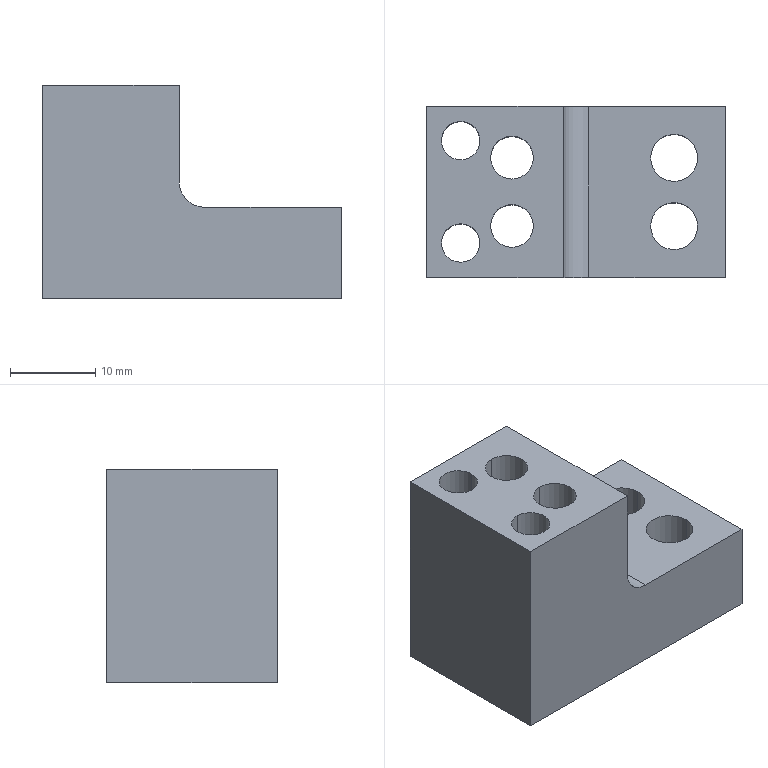Part | NX | 1 solid | 21 faces | box 35 x 20 x 25 mm | volume 9819 mm3 | cylinder 13 | plane 8 | commonest cylinder face diameters 4.5 x4 5 x4 5.5 x4 6 x1
STEP:
#1=CARTESIAN_POINT('',(0.,-20.,0.));
#2=VERTEX_POINT('',#1);
#3=CARTESIAN_POINT('',(0.,0.,0.));
#4=VERTEX_POINT('',#3);
#5=CARTESIAN_POINT('',(0.,0.,0.));
#6=DIRECTION('',(0.,1.,0.));
#7=VECTOR('',#6,1000.);
#8=LINE('',#5,#7);
#9=EDGE_CURVE('',#2,#4,#8,.T.);
#10=ORIENTED_EDGE('',*,*,#9,.T.);
#11=CARTESIAN_POINT('',(35.,0.,0.));
#12=VERTEX_POINT('',#11);
#13=CARTESIAN_POINT('',(0.,0.,0.));
#14=DIRECTION('',(1.,0.,0.));
#15=VECTOR('',#14,1000.);
#16=LINE('',#13,#15);
#17=EDGE_CURVE('',#4,#12,#16,.T.);
#18=ORIENTED_EDGE('',*,*,#17,.T.);
#19=CARTESIAN_POINT('',(35.,-20.,0.));
#20=VERTEX_POINT('',#19);
#21=CARTESIAN_POINT('',(35.,0.,0.));
#22=DIRECTION('',(0.,-1.,0.));
#23=VECTOR('',#22,1000.);
#24=LINE('',#21,#23);
#25=EDGE_CURVE('',#12,#20,#24,.T.);
#26=ORIENTED_EDGE('',*,*,#25,.T.);
#27=CARTESIAN_POINT('',(0.,-20.,0.));
#28=DIRECTION('',(-1.,0.,0.));
#29=VECTOR('',#28,1000.);
#30=LINE('',#27,#29);
#31=EDGE_CURVE('',#20,#2,#30,.T.);
#32=ORIENTED_EDGE('',*,*,#31,.T.);
#33=EDGE_LOOP('',(#10,#18,#26,#32));
#34=FACE_BOUND('',#33,.T.);
#35=CARTESIAN_POINT('',(6.25,-4.,0.));
#36=VERTEX_POINT('',#35);
#37=CARTESIAN_POINT('',(1.75,-4.,0.));
#38=VERTEX_POINT('',#37);
#39=CARTESIAN_POINT('',(4.,-4.,0.));
#40=DIRECTION('',(0.,0.,1.));
#41=DIRECTION('',(1.,0.,0.));
#42=AXIS2_PLACEMENT_3D('',#39,#40,#41);
#43=CIRCLE('',#42,2.25);
#44=EDGE_CURVE('',#36,#38,#43,.T.);
#45=ORIENTED_EDGE('',*,*,#44,.T.);
#46=CARTESIAN_POINT('',(4.,-4.,0.));
#47=DIRECTION('',(0.,0.,1.));
#48=DIRECTION('',(1.,0.,0.));
#49=AXIS2_PLACEMENT_3D('',#46,#47,#48);
#50=CIRCLE('',#49,2.25);
#51=EDGE_CURVE('',#38,#36,#50,.T.);
#52=ORIENTED_EDGE('',*,*,#51,.T.);
#53=EDGE_LOOP('',(#45,#52));
#54=FACE_BOUND('',#53,.T.);
#55=CARTESIAN_POINT('',(31.75,-14.,0.));
#56=VERTEX_POINT('',#55);
#57=CARTESIAN_POINT('',(26.25,-14.,0.));
#58=VERTEX_POINT('',#57);
#59=CARTESIAN_POINT('',(29.,-14.,0.));
#60=DIRECTION('',(0.,0.,-1.));
#61=DIRECTION('',(-1.,0.,0.));
#62=AXIS2_PLACEMENT_3D('',#59,#60,#61);
#63=CIRCLE('',#62,2.75);
#64=EDGE_CURVE('',#56,#58,#63,.T.);
#65=ORIENTED_EDGE('',*,*,#64,.F.);
#66=CARTESIAN_POINT('',(29.,-14.,0.));
#67=DIRECTION('',(0.,0.,-1.));
#68=DIRECTION('',(-1.,0.,0.));
#69=AXIS2_PLACEMENT_3D('',#66,#67,#68);
#70=CIRCLE('',#69,2.75);
#71=EDGE_CURVE('',#58,#56,#70,.T.);
#72=ORIENTED_EDGE('',*,*,#71,.F.);
#73=EDGE_LOOP('',(#65,#72));
#74=FACE_BOUND('',#73,.T.);
#75=CARTESIAN_POINT('',(31.75,-6.,0.));
#76=VERTEX_POINT('',#75);
#77=CARTESIAN_POINT('',(26.25,-6.,0.));
#78=VERTEX_POINT('',#77);
#79=CARTESIAN_POINT('',(29.,-6.,0.));
#80=DIRECTION('',(0.,0.,-1.));
#81=DIRECTION('',(-1.,0.,0.));
#82=AXIS2_PLACEMENT_3D('',#79,#80,#81);
#83=CIRCLE('',#82,2.75);
#84=EDGE_CURVE('',#76,#78,#83,.T.);
#85=ORIENTED_EDGE('',*,*,#84,.F.);
#86=CARTESIAN_POINT('',(29.,-6.,0.));
#87=DIRECTION('',(0.,0.,-1.));
#88=DIRECTION('',(-1.,0.,0.));
#89=AXIS2_PLACEMENT_3D('',#86,#87,#88);
#90=CIRCLE('',#89,2.75);
#91=EDGE_CURVE('',#78,#76,#90,.T.);
#92=ORIENTED_EDGE('',*,*,#91,.F.);
#93=EDGE_LOOP('',(#85,#92));
#94=FACE_BOUND('',#93,.T.);
#95=CARTESIAN_POINT('',(10.,-3.5,0.));
#96=VERTEX_POINT('',#95);
#97=CARTESIAN_POINT('',(10.,-8.5,0.));
#98=VERTEX_POINT('',#97);
#99=CARTESIAN_POINT('',(10.,-6.,0.));
#100=DIRECTION('',(0.,0.,-1.));
#101=DIRECTION('',(0.,1.,0.));
#102=AXIS2_PLACEMENT_3D('',#99,#100,#101);
#103=CIRCLE('',#102,2.5);
#104=EDGE_CURVE('',#96,#98,#103,.T.);
#105=ORIENTED_EDGE('',*,*,#104,.F.);
#106=CARTESIAN_POINT('',(10.,-6.,0.));
#107=DIRECTION('',(0.,0.,-1.));
#108=DIRECTION('',(0.,1.,0.));
#109=AXIS2_PLACEMENT_3D('',#106,#107,#108);
#110=CIRCLE('',#109,2.5);
#111=EDGE_CURVE('',#98,#96,#110,.T.);
#112=ORIENTED_EDGE('',*,*,#111,.F.);
#113=EDGE_LOOP('',(#105,#112));
#114=FACE_BOUND('',#113,.T.);
#115=CARTESIAN_POINT('',(10.,-16.5,0.));
#116=VERTEX_POINT('',#115);
#117=CARTESIAN_POINT('',(10.,-11.5,0.));
#118=VERTEX_POINT('',#117);
#119=CARTESIAN_POINT('',(10.,-14.,0.));
#120=DIRECTION('',(0.,0.,-1.));
#121=DIRECTION('',(0.,1.,0.));
#122=AXIS2_PLACEMENT_3D('',#119,#120,#121);
#123=CIRCLE('',#122,2.5);
#124=EDGE_CURVE('',#116,#118,#123,.T.);
#125=ORIENTED_EDGE('',*,*,#124,.F.);
#126=CARTESIAN_POINT('',(10.,-14.,0.));
#127=DIRECTION('',(0.,0.,-1.));
#128=DIRECTION('',(0.,1.,0.));
#129=AXIS2_PLACEMENT_3D('',#126,#127,#128);
#130=CIRCLE('',#129,2.5);
#131=EDGE_CURVE('',#118,#116,#130,.T.);
#132=ORIENTED_EDGE('',*,*,#131,.F.);
#133=EDGE_LOOP('',(#125,#132));
#134=FACE_BOUND('',#133,.T.);
#135=CARTESIAN_POINT('',(4.,-13.75,0.));
#136=VERTEX_POINT('',#135);
#137=CARTESIAN_POINT('',(4.,-18.25,0.));
#138=VERTEX_POINT('',#137);
#139=CARTESIAN_POINT('',(4.,-16.,0.));
#140=DIRECTION('',(0.,0.,-1.));
#141=DIRECTION('',(0.,1.,0.));
#142=AXIS2_PLACEMENT_3D('',#139,#140,#141);
#143=CIRCLE('',#142,2.25);
#144=EDGE_CURVE('',#136,#138,#143,.T.);
#145=ORIENTED_EDGE('',*,*,#144,.F.);
#146=CARTESIAN_POINT('',(4.,-16.,0.));
#147=DIRECTION('',(0.,0.,-1.));
#148=DIRECTION('',(0.,1.,0.));
#149=AXIS2_PLACEMENT_3D('',#146,#147,#148);
#150=CIRCLE('',#149,2.25);
#151=EDGE_CURVE('',#138,#136,#150,.T.);
#152=ORIENTED_EDGE('',*,*,#151,.F.);
#153=EDGE_LOOP('',(#145,#152));
#154=FACE_BOUND('',#153,.T.);
#155=CARTESIAN_POINT('',(0.,0.,0.));
#156=DIRECTION('',(0.,0.,1.));
#157=DIRECTION('',(1.,0.,0.));
#158=AXIS2_PLACEMENT_3D('',#155,#156,#157);
#159=PLANE('',#158);
#160=ADVANCED_FACE('',(#34,#54,#74,#94,#114,#134,#154),#159,.F.);
#161=ORIENTED_EDGE('',*,*,#9,.F.);
#162=CARTESIAN_POINT('',(0.,-20.,25.));
#163=VERTEX_POINT('',#162);
#164=CARTESIAN_POINT('',(0.,-20.,25.));
#165=DIRECTION('',(0.,0.,-1.));
#166=VECTOR('',#165,1000.);
#167=LINE('',#164,#166);
#168=EDGE_CURVE('',#163,#2,#167,.T.);
#169=ORIENTED_EDGE('',*,*,#168,.F.);
#170=CARTESIAN_POINT('',(0.,0.,25.));
#171=VERTEX_POINT('',#170);
#172=CARTESIAN_POINT('',(0.,0.,25.));
#173=DIRECTION('',(0.,1.,0.));
#174=VECTOR('',#173,1000.);
#175=LINE('',#172,#174);
#176=EDGE_CURVE('',#163,#171,#175,.T.);
#177=ORIENTED_EDGE('',*,*,#176,.T.);
#178=CARTESIAN_POINT('',(0.,0.,25.));
#179=DIRECTION('',(0.,0.,-1.));
#180=VECTOR('',#179,1000.);
#181=LINE('',#178,#180);
#182=EDGE_CURVE('',#171,#4,#181,.T.);
#183=ORIENTED_EDGE('',*,*,#182,.T.);
#184=EDGE_LOOP('',(#161,#169,#177,#183));
#185=FACE_BOUND('',#184,.T.);
#186=CARTESIAN_POINT('',(0.,0.,0.));
#187=DIRECTION('',(-1.,0.,0.));
#188=DIRECTION('',(0.,0.,1.));
#189=AXIS2_PLACEMENT_3D('',#186,#187,#188);
#190=PLANE('',#189);
#191=ADVANCED_FACE('',(#185),#190,.T.);
#192=CARTESIAN_POINT('',(19.,0.,10.7));
#193=VERTEX_POINT('',#192);
#194=CARTESIAN_POINT('',(35.,0.,10.7));
#195=VERTEX_POINT('',#194);
#196=CARTESIAN_POINT('',(19.,0.,10.7));
#197=DIRECTION('',(1.,0.,0.));
#198=VECTOR('',#197,1000.);
#199=LINE('',#196,#198);
#200=EDGE_CURVE('',#193,#195,#199,.T.);
#201=ORIENTED_EDGE('',*,*,#200,.T.);
#202=CARTESIAN_POINT('',(35.,0.,10.7));
#203=DIRECTION('',(0.,0.,-1.));
#204=VECTOR('',#203,1000.);
#205=LINE('',#202,#204);
#206=EDGE_CURVE('',#195,#12,#205,.T.);
#207=ORIENTED_EDGE('',*,*,#206,.T.);
#208=ORIENTED_EDGE('',*,*,#17,.F.);
#209=ORIENTED_EDGE('',*,*,#182,.F.);
#210=CARTESIAN_POINT('',(16.,0.,25.));
#211=VERTEX_POINT('',#210);
#212=CARTESIAN_POINT('',(0.,0.,25.));
#213=DIRECTION('',(1.,0.,0.));
#214=VECTOR('',#213,1000.);
#215=LINE('',#212,#214);
#216=EDGE_CURVE('',#171,#211,#215,.T.);
#217=ORIENTED_EDGE('',*,*,#216,.T.);
#218=CARTESIAN_POINT('',(16.,0.,13.7));
#219=VERTEX_POINT('',#218);
#220=CARTESIAN_POINT('',(16.,0.,13.7));
#221=DIRECTION('',(0.,0.,1.));
#222=VECTOR('',#221,1000.);
#223=LINE('',#220,#222);
#224=EDGE_CURVE('',#219,#211,#223,.T.);
#225=ORIENTED_EDGE('',*,*,#224,.F.);
#226=CARTESIAN_POINT('',(19.,0.,13.7));
#227=DIRECTION('',(0.,1.,0.));
#228=DIRECTION('',(0.,0.,-1.));
#229=AXIS2_PLACEMENT_3D('',#226,#227,#228);
#230=CIRCLE('',#229,3.);
#231=EDGE_CURVE('',#193,#219,#230,.T.);
#232=ORIENTED_EDGE('',*,*,#231,.F.);
#233=EDGE_LOOP('',(#201,#207,#208,#209,#217,#225,#232));
#234=FACE_BOUND('',#233,.T.);
#235=CARTESIAN_POINT('',(35.,0.,0.));
#236=DIRECTION('',(0.,1.,0.));
#237=DIRECTION('',(1.,0.,0.));
#238=AXIS2_PLACEMENT_3D('',#235,#236,#237);
#239=PLANE('',#238);
#240=ADVANCED_FACE('',(#234),#239,.T.);
#241=CARTESIAN_POINT('',(19.,-20.,10.7));
#242=VERTEX_POINT('',#241);
#243=CARTESIAN_POINT('',(19.,0.,10.7));
#244=DIRECTION('',(0.,-1.,0.));
#245=VECTOR('',#244,1000.);
#246=LINE('',#243,#245);
#247=EDGE_CURVE('',#193,#242,#246,.T.);
#248=ORIENTED_EDGE('',*,*,#247,.T.);
#249=CARTESIAN_POINT('',(35.,-20.,10.7));
#250=VERTEX_POINT('',#249);
#251=CARTESIAN_POINT('',(19.,-20.,10.7));
#252=DIRECTION('',(1.,0.,0.));
#253=VECTOR('',#252,1000.);
#254=LINE('',#251,#253);
#255=EDGE_CURVE('',#242,#250,#254,.T.);
#256=ORIENTED_EDGE('',*,*,#255,.T.);
#257=CARTESIAN_POINT('',(35.,0.,10.7));
#258=DIRECTION('',(0.,-1.,0.));
#259=VECTOR('',#258,1000.);
#260=LINE('',#257,#259);
#261=EDGE_CURVE('',#195,#250,#260,.T.);
#262=ORIENTED_EDGE('',*,*,#261,.F.);
#263=ORIENTED_EDGE('',*,*,#200,.F.);
#264=EDGE_LOOP('',(#248,#256,#262,#263));
#265=FACE_BOUND('',#264,.T.);
#266=CARTESIAN_POINT('',(31.75,-6.,10.7));
#267=VERTEX_POINT('',#266);
#268=CARTESIAN_POINT('',(26.25,-6.,10.7));
#269=VERTEX_POINT('',#268);
#270=CARTESIAN_POINT('',(29.,-6.,10.7));
#271=DIRECTION('',(0.,0.,1.));
#272=DIRECTION('',(-1.,0.,0.));
#273=AXIS2_PLACEMENT_3D('',#270,#271,#272);
#274=CIRCLE('',#273,2.75);
#275=EDGE_CURVE('',#267,#269,#274,.T.);
#276=ORIENTED_EDGE('',*,*,#275,.F.);
#277=CARTESIAN_POINT('',(29.,-6.,10.7));
#278=DIRECTION('',(0.,0.,1.));
#279=DIRECTION('',(-1.,0.,0.));
#280=AXIS2_PLACEMENT_3D('',#277,#278,#279);
#281=CIRCLE('',#280,2.75);
#282=EDGE_CURVE('',#269,#267,#281,.T.);
#283=ORIENTED_EDGE('',*,*,#282,.F.);
#284=EDGE_LOOP('',(#276,#283));
#285=FACE_BOUND('',#284,.T.);
#286=CARTESIAN_POINT('',(31.75,-14.,10.7));
#287=VERTEX_POINT('',#286);
#288=CARTESIAN_POINT('',(26.25,-14.,10.7));
#289=VERTEX_POINT('',#288);
#290=CARTESIAN_POINT('',(29.,-14.,10.7));
#291=DIRECTION('',(0.,0.,1.));
#292=DIRECTION('',(-1.,0.,0.));
#293=AXIS2_PLACEMENT_3D('',#290,#291,#292);
#294=CIRCLE('',#293,2.75);
#295=EDGE_CURVE('',#287,#289,#294,.T.);
#296=ORIENTED_EDGE('',*,*,#295,.F.);
#297=CARTESIAN_POINT('',(29.,-14.,10.7));
#298=DIRECTION('',(0.,0.,1.));
#299=DIRECTION('',(-1.,0.,0.));
#300=AXIS2_PLACEMENT_3D('',#297,#298,#299);
#301=CIRCLE('',#300,2.75);
#302=EDGE_CURVE('',#289,#287,#301,.T.);
#303=ORIENTED_EDGE('',*,*,#302,.F.);
#304=EDGE_LOOP('',(#296,#303));
#305=FACE_BOUND('',#304,.T.);
#306=CARTESIAN_POINT('',(35.,0.,10.7));
#307=DIRECTION('',(0.,0.,-1.));
#308=DIRECTION('',(0.,-1.,0.));
#309=AXIS2_PLACEMENT_3D('',#306,#307,#308);
#310=PLANE('',#309);
#311=ADVANCED_FACE('',(#265,#285,#305),#310,.F.);
#312=CARTESIAN_POINT('',(16.,-20.,13.7));
#313=VERTEX_POINT('',#312);
#314=CARTESIAN_POINT('',(16.,0.07422,13.7));
#315=DIRECTION('',(0.,-1.,0.));
#316=VECTOR('',#315,1000.);
#317=LINE('',#314,#316);
#318=EDGE_CURVE('',#219,#313,#317,.T.);
#319=ORIENTED_EDGE('',*,*,#318,.T.);
#320=CARTESIAN_POINT('',(19.,-20.,13.7));
#321=DIRECTION('',(0.,-1.,0.));
#322=DIRECTION('',(-1.,0.,0.));
#323=AXIS2_PLACEMENT_3D('',#320,#321,#322);
#324=CIRCLE('',#323,3.);
#325=EDGE_CURVE('',#313,#242,#324,.T.);
#326=ORIENTED_EDGE('',*,*,#325,.T.);
#327=ORIENTED_EDGE('',*,*,#247,.F.);
#328=ORIENTED_EDGE('',*,*,#231,.T.);
#329=EDGE_LOOP('',(#319,#326,#327,#328));
#330=FACE_BOUND('',#329,.T.);
#331=CARTESIAN_POINT('',(19.,0.07422,13.7));
#332=DIRECTION('',(0.,-1.,0.));
#333=DIRECTION('',(-1.,0.,0.));
#334=AXIS2_PLACEMENT_3D('',#331,#332,#333);
#335=CYLINDRICAL_SURFACE('',#334,3.);
#336=ADVANCED_FACE('',(#330),#335,.F.);
#337=ORIENTED_EDGE('',*,*,#318,.F.);
#338=ORIENTED_EDGE('',*,*,#224,.T.);
#339=CARTESIAN_POINT('',(16.,-20.,25.));
#340=VERTEX_POINT('',#339);
#341=CARTESIAN_POINT('',(16.,0.,25.));
#342=DIRECTION('',(0.,1.,0.));
#343=VECTOR('',#342,1000.);
#344=LINE('',#341,#343);
#345=EDGE_CURVE('',#340,#211,#344,.T.);
#346=ORIENTED_EDGE('',*,*,#345,.F.);
#347=CARTESIAN_POINT('',(16.,-20.,13.7));
#348=DIRECTION('',(0.,0.,1.));
#349=VECTOR('',#348,1000.);
#350=LINE('',#347,#349);
#351=EDGE_CURVE('',#313,#340,#350,.T.);
#352=ORIENTED_EDGE('',*,*,#351,.F.);
#353=EDGE_LOOP('',(#337,#338,#346,#352));
#354=FACE_BOUND('',#353,.T.);
#355=CARTESIAN_POINT('',(16.,0.,10.7));
#356=DIRECTION('',(-1.,0.,0.));
#357=DIRECTION('',(0.,0.,1.));
#358=AXIS2_PLACEMENT_3D('',#355,#356,#357);
#359=PLANE('',#358);
#360=ADVANCED_FACE('',(#354),#359,.F.);
#361=ORIENTED_EDGE('',*,*,#351,.T.);
#362=CARTESIAN_POINT('',(0.,-20.,25.));
#363=DIRECTION('',(-1.,0.,0.));
#364=VECTOR('',#363,1000.);
#365=LINE('',#362,#364);
#366=EDGE_CURVE('',#340,#163,#365,.T.);
#367=ORIENTED_EDGE('',*,*,#366,.T.);
#368=ORIENTED_EDGE('',*,*,#168,.T.);
#369=ORIENTED_EDGE('',*,*,#31,.F.);
#370=CARTESIAN_POINT('',(35.,-20.,10.7));
#371=DIRECTION('',(0.,0.,-1.));
#372=VECTOR('',#371,1000.);
#373=LINE('',#370,#372);
#374=EDGE_CURVE('',#250,#20,#373,.T.);
#375=ORIENTED_EDGE('',*,*,#374,.F.);
#376=ORIENTED_EDGE('',*,*,#255,.F.);
#377=ORIENTED_EDGE('',*,*,#325,.F.);
#378=EDGE_LOOP('',(#361,#367,#368,#369,#375,#376,#377));
#379=FACE_BOUND('',#378,.T.);
#380=CARTESIAN_POINT('',(0.,-20.,0.));
#381=DIRECTION('',(0.,-1.,0.));
#382=DIRECTION('',(0.,0.,-1.));
#383=AXIS2_PLACEMENT_3D('',#380,#381,#382);
#384=PLANE('',#383);
#385=ADVANCED_FACE('',(#379),#384,.T.);
#386=ORIENTED_EDGE('',*,*,#261,.T.);
#387=ORIENTED_EDGE('',*,*,#374,.T.);
#388=ORIENTED_EDGE('',*,*,#25,.F.);
#389=ORIENTED_EDGE('',*,*,#206,.F.);
#390=EDGE_LOOP('',(#386,#387,#388,#389));
#391=FACE_BOUND('',#390,.T.);
#392=CARTESIAN_POINT('',(35.,-20.,0.));
#393=DIRECTION('',(1.,0.,0.));
#394=DIRECTION('',(0.,1.,0.));
#395=AXIS2_PLACEMENT_3D('',#392,#393,#394);
#396=PLANE('',#395);
#397=ADVANCED_FACE('',(#391),#396,.T.);
#398=ORIENTED_EDGE('',*,*,#345,.T.);
#399=ORIENTED_EDGE('',*,*,#216,.F.);
#400=ORIENTED_EDGE('',*,*,#176,.F.);
#401=ORIENTED_EDGE('',*,*,#366,.F.);
#402=EDGE_LOOP('',(#398,#399,#400,#401));
#403=FACE_BOUND('',#402,.T.);
#404=CARTESIAN_POINT('',(1.75,-4.,25.));
#405=VERTEX_POINT('',#404);
#406=CARTESIAN_POINT('',(6.25,-4.,25.));
#407=VERTEX_POINT('',#406);
#408=CARTESIAN_POINT('',(4.,-4.,25.));
#409=DIRECTION('',(0.,0.,1.));
#410=DIRECTION('',(1.,0.,0.));
#411=AXIS2_PLACEMENT_3D('',#408,#409,#410);
#412=CIRCLE('',#411,2.25);
#413=EDGE_CURVE('',#405,#407,#412,.T.);
#414=ORIENTED_EDGE('',*,*,#413,.F.);
#415=CARTESIAN_POINT('',(4.,-4.,25.));
#416=DIRECTION('',(0.,0.,1.));
#417=DIRECTION('',(1.,0.,0.));
#418=AXIS2_PLACEMENT_3D('',#415,#416,#417);
#419=CIRCLE('',#418,2.25);
#420=EDGE_CURVE('',#407,#405,#419,.T.);
#421=ORIENTED_EDGE('',*,*,#420,.F.);
#422=EDGE_LOOP('',(#414,#421));
#423=FACE_BOUND('',#422,.T.);
#424=CARTESIAN_POINT('',(4.,-18.25,25.));
#425=VERTEX_POINT('',#424);
#426=CARTESIAN_POINT('',(4.,-13.75,25.));
#427=VERTEX_POINT('',#426);
#428=CARTESIAN_POINT('',(4.,-16.,25.));
#429=DIRECTION('',(0.,0.,-1.));
#430=DIRECTION('',(0.,1.,0.));
#431=AXIS2_PLACEMENT_3D('',#428,#429,#430);
#432=CIRCLE('',#431,2.25);
#433=EDGE_CURVE('',#425,#427,#432,.T.);
#434=ORIENTED_EDGE('',*,*,#433,.T.);
#435=CARTESIAN_POINT('',(4.,-16.,25.));
#436=DIRECTION('',(0.,0.,-1.));
#437=DIRECTION('',(0.,1.,0.));
#438=AXIS2_PLACEMENT_3D('',#435,#436,#437);
#439=CIRCLE('',#438,2.25);
#440=EDGE_CURVE('',#427,#425,#439,.T.);
#441=ORIENTED_EDGE('',*,*,#440,.T.);
#442=EDGE_LOOP('',(#434,#441));
#443=FACE_BOUND('',#442,.T.);
#444=CARTESIAN_POINT('',(10.,-11.5,25.));
#445=VERTEX_POINT('',#444);
#446=CARTESIAN_POINT('',(10.,-16.5,25.));
#447=VERTEX_POINT('',#446);
#448=CARTESIAN_POINT('',(10.,-14.,25.));
#449=DIRECTION('',(0.,0.,-1.));
#450=DIRECTION('',(0.,1.,0.));
#451=AXIS2_PLACEMENT_3D('',#448,#449,#450);
#452=CIRCLE('',#451,2.5);
#453=EDGE_CURVE('',#445,#447,#452,.T.);
#454=ORIENTED_EDGE('',*,*,#453,.T.);
#455=CARTESIAN_POINT('',(10.,-14.,25.));
#456=DIRECTION('',(0.,0.,-1.));
#457=DIRECTION('',(0.,1.,0.));
#458=AXIS2_PLACEMENT_3D('',#455,#456,#457);
#459=CIRCLE('',#458,2.5);
#460=EDGE_CURVE('',#447,#445,#459,.T.);
#461=ORIENTED_EDGE('',*,*,#460,.T.);
#462=EDGE_LOOP('',(#454,#461));
#463=FACE_BOUND('',#462,.T.);
#464=CARTESIAN_POINT('',(10.,-3.5,25.));
#465=VERTEX_POINT('',#464);
#466=CARTESIAN_POINT('',(10.,-8.5,25.));
#467=VERTEX_POINT('',#466);
#468=CARTESIAN_POINT('',(10.,-6.,25.));
#469=DIRECTION('',(0.,0.,-1.));
#470=DIRECTION('',(0.,1.,0.));
#471=AXIS2_PLACEMENT_3D('',#468,#469,#470);
#472=CIRCLE('',#471,2.5);
#473=EDGE_CURVE('',#465,#467,#472,.T.);
#474=ORIENTED_EDGE('',*,*,#473,.T.);
#475=CARTESIAN_POINT('',(10.,-6.,25.));
#476=DIRECTION('',(0.,0.,-1.));
#477=DIRECTION('',(0.,1.,0.));
#478=AXIS2_PLACEMENT_3D('',#475,#476,#477);
#479=CIRCLE('',#478,2.5);
#480=EDGE_CURVE('',#467,#465,#479,.T.);
#481=ORIENTED_EDGE('',*,*,#480,.T.);
#482=EDGE_LOOP('',(#474,#481));
#483=FACE_BOUND('',#482,.T.);
#484=CARTESIAN_POINT('',(0.,0.,25.));
#485=DIRECTION('',(0.,0.,1.));
#486=DIRECTION('',(1.,0.,0.));
#487=AXIS2_PLACEMENT_3D('',#484,#485,#486);
#488=PLANE('',#487);
#489=ADVANCED_FACE('',(#403,#423,#443,#463,#483),#488,.T.);
#490=ORIENTED_EDGE('',*,*,#44,.F.);
#491=CARTESIAN_POINT('',(6.25,-4.,0.));
#492=DIRECTION('',(0.,0.,1.));
#493=VECTOR('',#492,1000.);
#494=LINE('',#491,#493);
#495=EDGE_CURVE('',#36,#407,#494,.T.);
#496=ORIENTED_EDGE('',*,*,#495,.T.);
#497=ORIENTED_EDGE('',*,*,#420,.T.);
#498=CARTESIAN_POINT('',(1.75,-4.,0.));
#499=DIRECTION('',(0.,0.,1.));
#500=VECTOR('',#499,1000.);
#501=LINE('',#498,#500);
#502=EDGE_CURVE('',#38,#405,#501,.T.);
#503=ORIENTED_EDGE('',*,*,#502,.F.);
#504=EDGE_LOOP('',(#490,#496,#497,#503));
#505=FACE_BOUND('',#504,.T.);
#506=CARTESIAN_POINT('',(4.,-4.,0.));
#507=DIRECTION('',(0.,0.,1.));
#508=DIRECTION('',(1.,0.,0.));
#509=AXIS2_PLACEMENT_3D('',#506,#507,#508);
#510=CYLINDRICAL_SURFACE('',#509,2.25);
#511=ADVANCED_FACE('',(#505),#510,.F.);
#512=ORIENTED_EDGE('',*,*,#84,.T.);
#513=CARTESIAN_POINT('',(26.25,-6.,25.));
#514=DIRECTION('',(0.,0.,-1.));
#515=VECTOR('',#514,1000.);
#516=LINE('',#513,#515);
#517=EDGE_CURVE('',#78,#269,#516,.F.);
#518=ORIENTED_EDGE('',*,*,#517,.T.);
#519=ORIENTED_EDGE('',*,*,#282,.T.);
#520=CARTESIAN_POINT('',(31.75,-6.,25.));
#521=DIRECTION('',(0.,0.,-1.));
#522=VECTOR('',#521,1000.);
#523=LINE('',#520,#522);
#524=EDGE_CURVE('',#76,#267,#523,.F.);
#525=ORIENTED_EDGE('',*,*,#524,.F.);
#526=EDGE_LOOP('',(#512,#518,#519,#525));
#527=FACE_BOUND('',#526,.T.);
#528=CARTESIAN_POINT('',(29.,-6.,25.));
#529=DIRECTION('',(0.,0.,-1.));
#530=DIRECTION('',(-1.,0.,0.));
#531=AXIS2_PLACEMENT_3D('',#528,#529,#530);
#532=CYLINDRICAL_SURFACE('',#531,2.75);
#533=ADVANCED_FACE('',(#527),#532,.F.);
#534=ORIENTED_EDGE('',*,*,#64,.T.);
#535=CARTESIAN_POINT('',(26.25,-14.,25.));
#536=DIRECTION('',(0.,0.,-1.));
#537=VECTOR('',#536,1000.);
#538=LINE('',#535,#537);
#539=EDGE_CURVE('',#58,#289,#538,.F.);
#540=ORIENTED_EDGE('',*,*,#539,.T.);
#541=ORIENTED_EDGE('',*,*,#302,.T.);
#542=CARTESIAN_POINT('',(31.75,-14.,25.));
#543=DIRECTION('',(0.,0.,-1.));
#544=VECTOR('',#543,1000.);
#545=LINE('',#542,#544);
#546=EDGE_CURVE('',#56,#287,#545,.F.);
#547=ORIENTED_EDGE('',*,*,#546,.F.);
#548=EDGE_LOOP('',(#534,#540,#541,#547));
#549=FACE_BOUND('',#548,.T.);
#550=CARTESIAN_POINT('',(29.,-14.,25.));
#551=DIRECTION('',(0.,0.,-1.));
#552=DIRECTION('',(-1.,0.,0.));
#553=AXIS2_PLACEMENT_3D('',#550,#551,#552);
#554=CYLINDRICAL_SURFACE('',#553,2.75);
#555=ADVANCED_FACE('',(#549),#554,.F.);
#556=ORIENTED_EDGE('',*,*,#144,.T.);
#557=CARTESIAN_POINT('',(4.,-18.25,27.5));
#558=DIRECTION('',(0.,0.,-1.));
#559=VECTOR('',#558,1000.);
#560=LINE('',#557,#559);
#561=EDGE_CURVE('',#138,#425,#560,.F.);
#562=ORIENTED_EDGE('',*,*,#561,.T.);
#563=ORIENTED_EDGE('',*,*,#440,.F.);
#564=CARTESIAN_POINT('',(4.,-13.75,27.5));
#565=DIRECTION('',(0.,0.,-1.));
#566=VECTOR('',#565,1000.);
#567=LINE('',#564,#566);
#568=EDGE_CURVE('',#136,#427,#567,.F.);
#569=ORIENTED_EDGE('',*,*,#568,.F.);
#570=EDGE_LOOP('',(#556,#562,#563,#569));
#571=FACE_BOUND('',#570,.T.);
#572=CARTESIAN_POINT('',(4.,-16.,27.5));
#573=DIRECTION('',(0.,0.,-1.));
#574=DIRECTION('',(0.,1.,0.));
#575=AXIS2_PLACEMENT_3D('',#572,#573,#574);
#576=CYLINDRICAL_SURFACE('',#575,2.25);
#577=ADVANCED_FACE('',(#571),#576,.F.);
#578=ORIENTED_EDGE('',*,*,#453,.F.);
#579=CARTESIAN_POINT('',(10.,-11.5,27.5));
#580=DIRECTION('',(0.,0.,-1.));
#581=VECTOR('',#580,1000.);
#582=LINE('',#579,#581);
#583=EDGE_CURVE('',#445,#118,#582,.T.);
#584=ORIENTED_EDGE('',*,*,#583,.T.);
#585=ORIENTED_EDGE('',*,*,#131,.T.);
#586=CARTESIAN_POINT('',(10.,-16.5,27.5));
#587=DIRECTION('',(0.,0.,-1.));
#588=VECTOR('',#587,1000.);
#589=LINE('',#586,#588);
#590=EDGE_CURVE('',#447,#116,#589,.T.);
#591=ORIENTED_EDGE('',*,*,#590,.F.);
#592=EDGE_LOOP('',(#578,#584,#585,#591));
#593=FACE_BOUND('',#592,.T.);
#594=CARTESIAN_POINT('',(10.,-14.,27.5));
#595=DIRECTION('',(0.,0.,-1.));
#596=DIRECTION('',(0.,1.,0.));
#597=AXIS2_PLACEMENT_3D('',#594,#595,#596);
#598=CYLINDRICAL_SURFACE('',#597,2.5);
#599=ADVANCED_FACE('',(#593),#598,.F.);
#600=ORIENTED_EDGE('',*,*,#473,.F.);
#601=CARTESIAN_POINT('',(10.,-3.5,27.5));
#602=DIRECTION('',(0.,0.,-1.));
#603=VECTOR('',#602,1000.);
#604=LINE('',#601,#603);
#605=EDGE_CURVE('',#465,#96,#604,.T.);
#606=ORIENTED_EDGE('',*,*,#605,.T.);
#607=ORIENTED_EDGE('',*,*,#104,.T.);
#608=CARTESIAN_POINT('',(10.,-8.5,27.5));
#609=DIRECTION('',(0.,0.,-1.));
#610=VECTOR('',#609,1000.);
#611=LINE('',#608,#610);
#612=EDGE_CURVE('',#467,#98,#611,.T.);
#613=ORIENTED_EDGE('',*,*,#612,.F.);
#614=EDGE_LOOP('',(#600,#606,#607,#613));
#615=FACE_BOUND('',#614,.T.);
#616=CARTESIAN_POINT('',(10.,-6.,27.5));
#617=DIRECTION('',(0.,0.,-1.));
#618=DIRECTION('',(0.,1.,0.));
#619=AXIS2_PLACEMENT_3D('',#616,#617,#618);
#620=CYLINDRICAL_SURFACE('',#619,2.5);
#621=ADVANCED_FACE('',(#615),#620,.F.);
#622=ORIENTED_EDGE('',*,*,#605,.F.);
#623=ORIENTED_EDGE('',*,*,#480,.F.);
#624=ORIENTED_EDGE('',*,*,#612,.T.);
#625=ORIENTED_EDGE('',*,*,#111,.T.);
#626=EDGE_LOOP('',(#622,#623,#624,#625));
#627=FACE_BOUND('',#626,.T.);
#628=CARTESIAN_POINT('',(10.,-6.,27.5));
#629=DIRECTION('',(0.,0.,-1.));
#630=DIRECTION('',(0.,1.,0.));
#631=AXIS2_PLACEMENT_3D('',#628,#629,#630);
#632=CYLINDRICAL_SURFACE('',#631,2.5);
#633=ADVANCED_FACE('',(#627),#632,.F.);
#634=ORIENTED_EDGE('',*,*,#124,.T.);
#635=ORIENTED_EDGE('',*,*,#583,.F.);
#636=ORIENTED_EDGE('',*,*,#460,.F.);
#637=ORIENTED_EDGE('',*,*,#590,.T.);
#638=EDGE_LOOP('',(#634,#635,#636,#637));
#639=FACE_BOUND('',#638,.T.);
#640=CARTESIAN_POINT('',(10.,-14.,27.5));
#641=DIRECTION('',(0.,0.,-1.));
#642=DIRECTION('',(0.,1.,0.));
#643=AXIS2_PLACEMENT_3D('',#640,#641,#642);
#644=CYLINDRICAL_SURFACE('',#643,2.5);
#645=ADVANCED_FACE('',(#639),#644,.F.);
#646=ORIENTED_EDGE('',*,*,#295,.T.);
#647=ORIENTED_EDGE('',*,*,#539,.F.);
#648=ORIENTED_EDGE('',*,*,#71,.T.);
#649=ORIENTED_EDGE('',*,*,#546,.T.);
#650=EDGE_LOOP('',(#646,#647,#648,#649));
#651=FACE_BOUND('',#650,.T.);
#652=CARTESIAN_POINT('',(29.,-14.,25.));
#653=DIRECTION('',(0.,0.,-1.));
#654=DIRECTION('',(-1.,0.,0.));
#655=AXIS2_PLACEMENT_3D('',#652,#653,#654);
#656=CYLINDRICAL_SURFACE('',#655,2.75);
#657=ADVANCED_FACE('',(#651),#656,.F.);
#658=ORIENTED_EDGE('',*,*,#433,.F.);
#659=ORIENTED_EDGE('',*,*,#561,.F.);
#660=ORIENTED_EDGE('',*,*,#151,.T.);
#661=ORIENTED_EDGE('',*,*,#568,.T.);
#662=EDGE_LOOP('',(#658,#659,#660,#661));
#663=FACE_BOUND('',#662,.T.);
#664=CARTESIAN_POINT('',(4.,-16.,27.5));
#665=DIRECTION('',(0.,0.,-1.));
#666=DIRECTION('',(0.,1.,0.));
#667=AXIS2_PLACEMENT_3D('',#664,#665,#666);
#668=CYLINDRICAL_SURFACE('',#667,2.25);
#669=ADVANCED_FACE('',(#663),#668,.F.);
#670=ORIENTED_EDGE('',*,*,#275,.T.);
#671=ORIENTED_EDGE('',*,*,#517,.F.);
#672=ORIENTED_EDGE('',*,*,#91,.T.);
#673=ORIENTED_EDGE('',*,*,#524,.T.);
#674=EDGE_LOOP('',(#670,#671,#672,#673));
#675=FACE_BOUND('',#674,.T.);
#676=CARTESIAN_POINT('',(29.,-6.,25.));
#677=DIRECTION('',(0.,0.,-1.));
#678=DIRECTION('',(-1.,0.,0.));
#679=AXIS2_PLACEMENT_3D('',#676,#677,#678);
#680=CYLINDRICAL_SURFACE('',#679,2.75);
#681=ADVANCED_FACE('',(#675),#680,.F.);
#682=ORIENTED_EDGE('',*,*,#413,.T.);
#683=ORIENTED_EDGE('',*,*,#495,.F.);
#684=ORIENTED_EDGE('',*,*,#51,.F.);
#685=ORIENTED_EDGE('',*,*,#502,.T.);
#686=EDGE_LOOP('',(#682,#683,#684,#685));
#687=FACE_BOUND('',#686,.T.);
#688=CARTESIAN_POINT('',(4.,-4.,0.));
#689=DIRECTION('',(0.,0.,1.));
#690=DIRECTION('',(1.,0.,0.));
#691=AXIS2_PLACEMENT_3D('',#688,#689,#690);
#692=CYLINDRICAL_SURFACE('',#691,2.25);
#693=ADVANCED_FACE('',(#687),#692,.F.);
#694=CLOSED_SHELL('',(#160,#191,#240,#311,#336,#360,#385,#397,#489,#511,#533,#555,#577,#599,#621,#633,#645,#657,#669,#681,#693));
#695=MANIFOLD_SOLID_BREP('',#694);
#696=(LENGTH_UNIT()NAMED_UNIT(*)SI_UNIT(.MILLI.,.METRE.));
#697=UNCERTAINTY_MEASURE_WITH_UNIT(LENGTH_MEASURE(0.00001),#696,'','');
#698=(NAMED_UNIT(*)PLANE_ANGLE_UNIT()SI_UNIT($,.RADIAN.));
#699=(NAMED_UNIT(*)SI_UNIT($,.STERADIAN.)SOLID_ANGLE_UNIT());
#700=(GEOMETRIC_REPRESENTATION_CONTEXT(3)GLOBAL_UNCERTAINTY_ASSIGNED_CONTEXT((#697))GLOBAL_UNIT_ASSIGNED_CONTEXT((#696,#698,#699))REPRESENTATION_CONTEXT('',''));
#701=ADVANCED_BREP_SHAPE_REPRESENTATION('',(#695),#700);